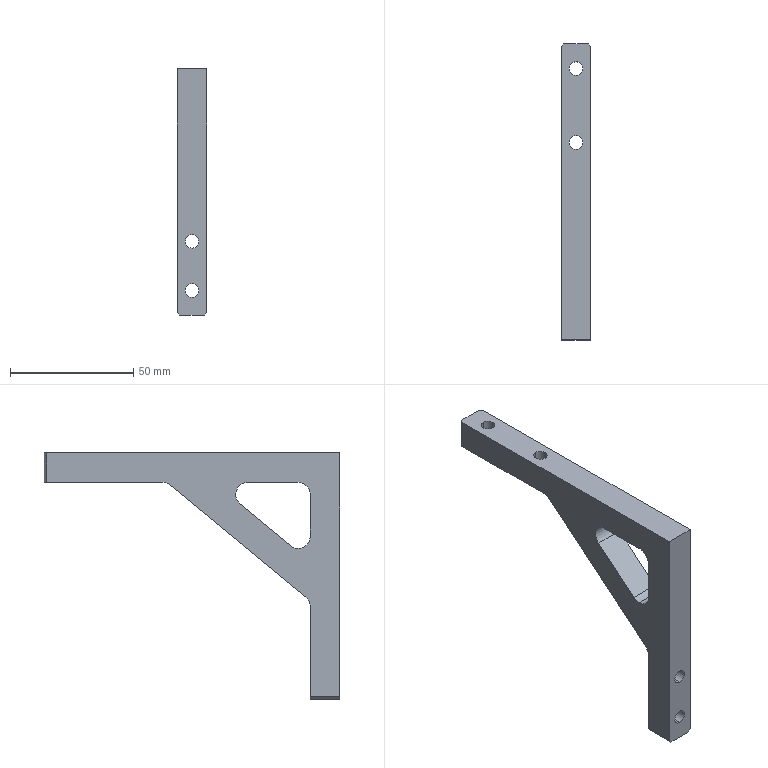Part | SolidWorks | features HoleWzd 2, Chamfer 1, Extrusion 1, Fillet 1, ICE 1 | 1 solid | 42 faces | box 12 x 120 x 100 mm | volume 37463 mm3 | cylinder 22 | plane 20 | commonest cylinder face diameters 10 x14 5.5 x8
STEP:
#1=CARTESIAN_POINT('',(6.,6.3,-95.));
#2=VERTEX_POINT('',#1);
#3=CARTESIAN_POINT('',(6.,6.3,-85.));
#4=VERTEX_POINT('',#3);
#5=CARTESIAN_POINT('',(6.,6.3,-90.));
#6=DIRECTION('',(0.,1.,0.));
#7=DIRECTION('',(0.,0.,1.));
#8=AXIS2_PLACEMENT_3D('',#5,#6,#7);
#9=CIRCLE('',#8,5.);
#10=EDGE_CURVE('',#2,#4,#9,.T.);
#11=ORIENTED_EDGE('',*,*,#10,.F.);
#12=CARTESIAN_POINT('',(6.,12.,-95.));
#13=VERTEX_POINT('',#12);
#14=CARTESIAN_POINT('',(6.,12.,-95.));
#15=DIRECTION('',(0.,1.,0.));
#16=VECTOR('',#15,1000.);
#17=LINE('',#14,#16);
#18=EDGE_CURVE('',#2,#13,#17,.T.);
#19=ORIENTED_EDGE('',*,*,#18,.T.);
#20=CARTESIAN_POINT('',(6.,12.,-85.));
#21=VERTEX_POINT('',#20);
#22=CARTESIAN_POINT('',(6.,12.,-90.));
#23=DIRECTION('',(0.,1.,0.));
#24=DIRECTION('',(0.,0.,1.));
#25=AXIS2_PLACEMENT_3D('',#22,#23,#24);
#26=CIRCLE('',#25,5.);
#27=EDGE_CURVE('',#13,#21,#26,.T.);
#28=ORIENTED_EDGE('',*,*,#27,.T.);
#29=CARTESIAN_POINT('',(6.,12.,-85.));
#30=DIRECTION('',(0.,1.,0.));
#31=VECTOR('',#30,1000.);
#32=LINE('',#29,#31);
#33=EDGE_CURVE('',#4,#21,#32,.T.);
#34=ORIENTED_EDGE('',*,*,#33,.F.);
#35=EDGE_LOOP('',(#11,#19,#28,#34));
#36=FACE_OUTER_BOUND('',#35,.T.);
#37=CARTESIAN_POINT('',(6.,12.,-90.));
#38=DIRECTION('',(0.,1.,0.));
#39=DIRECTION('',(0.,0.,1.));
#40=AXIS2_PLACEMENT_3D('',#37,#38,#39);
#41=CYLINDRICAL_SURFACE('',#40,5.);
#42=ADVANCED_FACE('',(#36),#41,.F.);
#43=CARTESIAN_POINT('',(6.,0.,-92.75));
#44=VERTEX_POINT('',#43);
#45=CARTESIAN_POINT('',(6.,0.,-87.25));
#46=VERTEX_POINT('',#45);
#47=CARTESIAN_POINT('',(6.,0.,-90.));
#48=DIRECTION('',(0.,1.,0.));
#49=DIRECTION('',(0.,0.,1.));
#50=AXIS2_PLACEMENT_3D('',#47,#48,#49);
#51=CIRCLE('',#50,2.75);
#52=EDGE_CURVE('',#44,#46,#51,.T.);
#53=ORIENTED_EDGE('',*,*,#52,.F.);
#54=CARTESIAN_POINT('',(6.,6.3,-92.75));
#55=VERTEX_POINT('',#54);
#56=CARTESIAN_POINT('',(6.,12.,-92.75));
#57=DIRECTION('',(0.,1.,0.));
#58=VECTOR('',#57,1000.);
#59=LINE('',#56,#58);
#60=EDGE_CURVE('',#44,#55,#59,.T.);
#61=ORIENTED_EDGE('',*,*,#60,.T.);
#62=CARTESIAN_POINT('',(6.,6.3,-87.25));
#63=VERTEX_POINT('',#62);
#64=CARTESIAN_POINT('',(6.,6.3,-90.));
#65=DIRECTION('',(0.,1.,0.));
#66=DIRECTION('',(0.,0.,1.));
#67=AXIS2_PLACEMENT_3D('',#64,#65,#66);
#68=CIRCLE('',#67,2.75);
#69=EDGE_CURVE('',#55,#63,#68,.T.);
#70=ORIENTED_EDGE('',*,*,#69,.T.);
#71=CARTESIAN_POINT('',(6.,12.,-87.25));
#72=DIRECTION('',(0.,1.,0.));
#73=VECTOR('',#72,1000.);
#74=LINE('',#71,#73);
#75=EDGE_CURVE('',#46,#63,#74,.T.);
#76=ORIENTED_EDGE('',*,*,#75,.F.);
#77=EDGE_LOOP('',(#53,#61,#70,#76));
#78=FACE_OUTER_BOUND('',#77,.T.);
#79=CARTESIAN_POINT('',(6.,12.,-90.));
#80=DIRECTION('',(0.,1.,0.));
#81=DIRECTION('',(0.,0.,1.));
#82=AXIS2_PLACEMENT_3D('',#79,#80,#81);
#83=CYLINDRICAL_SURFACE('',#82,2.75);
#84=ADVANCED_FACE('',(#78),#83,.F.);
#85=CARTESIAN_POINT('',(6.,6.3,-75.));
#86=VERTEX_POINT('',#85);
#87=CARTESIAN_POINT('',(6.,6.3,-65.));
#88=VERTEX_POINT('',#87);
#89=CARTESIAN_POINT('',(6.,6.3,-70.));
#90=DIRECTION('',(0.,1.,0.));
#91=DIRECTION('',(0.,0.,1.));
#92=AXIS2_PLACEMENT_3D('',#89,#90,#91);
#93=CIRCLE('',#92,5.);
#94=EDGE_CURVE('',#86,#88,#93,.T.);
#95=ORIENTED_EDGE('',*,*,#94,.F.);
#96=CARTESIAN_POINT('',(6.,12.,-75.));
#97=VERTEX_POINT('',#96);
#98=CARTESIAN_POINT('',(6.,12.,-75.));
#99=DIRECTION('',(0.,1.,0.));
#100=VECTOR('',#99,1000.);
#101=LINE('',#98,#100);
#102=EDGE_CURVE('',#86,#97,#101,.T.);
#103=ORIENTED_EDGE('',*,*,#102,.T.);
#104=CARTESIAN_POINT('',(6.,12.,-65.));
#105=VERTEX_POINT('',#104);
#106=CARTESIAN_POINT('',(6.,12.,-70.));
#107=DIRECTION('',(0.,1.,0.));
#108=DIRECTION('',(0.,0.,1.));
#109=AXIS2_PLACEMENT_3D('',#106,#107,#108);
#110=CIRCLE('',#109,5.);
#111=EDGE_CURVE('',#97,#105,#110,.T.);
#112=ORIENTED_EDGE('',*,*,#111,.T.);
#113=CARTESIAN_POINT('',(6.,12.,-65.));
#114=DIRECTION('',(0.,1.,0.));
#115=VECTOR('',#114,1000.);
#116=LINE('',#113,#115);
#117=EDGE_CURVE('',#88,#105,#116,.T.);
#118=ORIENTED_EDGE('',*,*,#117,.F.);
#119=EDGE_LOOP('',(#95,#103,#112,#118));
#120=FACE_OUTER_BOUND('',#119,.T.);
#121=CARTESIAN_POINT('',(6.,12.,-70.));
#122=DIRECTION('',(0.,1.,0.));
#123=DIRECTION('',(0.,0.,1.));
#124=AXIS2_PLACEMENT_3D('',#121,#122,#123);
#125=CYLINDRICAL_SURFACE('',#124,5.);
#126=ADVANCED_FACE('',(#120),#125,.F.);
#127=CARTESIAN_POINT('',(6.,0.,-72.75));
#128=VERTEX_POINT('',#127);
#129=CARTESIAN_POINT('',(6.,0.,-67.25));
#130=VERTEX_POINT('',#129);
#131=CARTESIAN_POINT('',(6.,0.,-70.));
#132=DIRECTION('',(0.,1.,0.));
#133=DIRECTION('',(0.,0.,1.));
#134=AXIS2_PLACEMENT_3D('',#131,#132,#133);
#135=CIRCLE('',#134,2.75);
#136=EDGE_CURVE('',#128,#130,#135,.T.);
#137=ORIENTED_EDGE('',*,*,#136,.F.);
#138=CARTESIAN_POINT('',(6.,6.3,-72.75));
#139=VERTEX_POINT('',#138);
#140=CARTESIAN_POINT('',(6.,12.,-72.75));
#141=DIRECTION('',(0.,1.,0.));
#142=VECTOR('',#141,1000.);
#143=LINE('',#140,#142);
#144=EDGE_CURVE('',#128,#139,#143,.T.);
#145=ORIENTED_EDGE('',*,*,#144,.T.);
#146=CARTESIAN_POINT('',(6.,6.3,-67.25));
#147=VERTEX_POINT('',#146);
#148=CARTESIAN_POINT('',(6.,6.3,-70.));
#149=DIRECTION('',(0.,1.,0.));
#150=DIRECTION('',(0.,0.,1.));
#151=AXIS2_PLACEMENT_3D('',#148,#149,#150);
#152=CIRCLE('',#151,2.75);
#153=EDGE_CURVE('',#139,#147,#152,.T.);
#154=ORIENTED_EDGE('',*,*,#153,.T.);
#155=CARTESIAN_POINT('',(6.,12.,-67.25));
#156=DIRECTION('',(0.,1.,0.));
#157=VECTOR('',#156,1000.);
#158=LINE('',#155,#157);
#159=EDGE_CURVE('',#130,#147,#158,.T.);
#160=ORIENTED_EDGE('',*,*,#159,.F.);
#161=EDGE_LOOP('',(#137,#145,#154,#160));
#162=FACE_OUTER_BOUND('',#161,.T.);
#163=CARTESIAN_POINT('',(6.,12.,-70.));
#164=DIRECTION('',(0.,1.,0.));
#165=DIRECTION('',(0.,0.,1.));
#166=AXIS2_PLACEMENT_3D('',#163,#164,#165);
#167=CYLINDRICAL_SURFACE('',#166,2.75);
#168=ADVANCED_FACE('',(#162),#167,.F.);
#169=CARTESIAN_POINT('',(6.,105.,-6.3));
#170=VERTEX_POINT('',#169);
#171=CARTESIAN_POINT('',(6.,115.,-6.3));
#172=VERTEX_POINT('',#171);
#173=CARTESIAN_POINT('',(6.,110.,-6.3));
#174=DIRECTION('',(0.,0.,-1.));
#175=DIRECTION('',(0.,1.,0.));
#176=AXIS2_PLACEMENT_3D('',#173,#174,#175);
#177=CIRCLE('',#176,5.);
#178=EDGE_CURVE('',#170,#172,#177,.T.);
#179=ORIENTED_EDGE('',*,*,#178,.F.);
#180=CARTESIAN_POINT('',(6.,105.,-12.));
#181=VERTEX_POINT('',#180);
#182=CARTESIAN_POINT('',(6.,105.,-12.));
#183=DIRECTION('',(0.,0.,-1.));
#184=VECTOR('',#183,1000.);
#185=LINE('',#182,#184);
#186=EDGE_CURVE('',#170,#181,#185,.T.);
#187=ORIENTED_EDGE('',*,*,#186,.T.);
#188=CARTESIAN_POINT('',(6.,115.,-12.));
#189=VERTEX_POINT('',#188);
#190=CARTESIAN_POINT('',(6.,110.,-12.));
#191=DIRECTION('',(0.,0.,-1.));
#192=DIRECTION('',(0.,1.,0.));
#193=AXIS2_PLACEMENT_3D('',#190,#191,#192);
#194=CIRCLE('',#193,5.);
#195=EDGE_CURVE('',#181,#189,#194,.T.);
#196=ORIENTED_EDGE('',*,*,#195,.T.);
#197=CARTESIAN_POINT('',(6.,115.,-12.));
#198=DIRECTION('',(0.,0.,-1.));
#199=VECTOR('',#198,1000.);
#200=LINE('',#197,#199);
#201=EDGE_CURVE('',#172,#189,#200,.T.);
#202=ORIENTED_EDGE('',*,*,#201,.F.);
#203=EDGE_LOOP('',(#179,#187,#196,#202));
#204=FACE_OUTER_BOUND('',#203,.T.);
#205=CARTESIAN_POINT('',(6.,110.,-12.));
#206=DIRECTION('',(0.,0.,-1.));
#207=DIRECTION('',(0.,1.,0.));
#208=AXIS2_PLACEMENT_3D('',#205,#206,#207);
#209=CYLINDRICAL_SURFACE('',#208,5.);
#210=ADVANCED_FACE('',(#204),#209,.F.);
#211=CARTESIAN_POINT('',(6.,107.25,0.));
#212=VERTEX_POINT('',#211);
#213=CARTESIAN_POINT('',(6.,112.75,0.));
#214=VERTEX_POINT('',#213);
#215=CARTESIAN_POINT('',(6.,110.,0.));
#216=DIRECTION('',(0.,0.,-1.));
#217=DIRECTION('',(0.,1.,0.));
#218=AXIS2_PLACEMENT_3D('',#215,#216,#217);
#219=CIRCLE('',#218,2.75);
#220=EDGE_CURVE('',#212,#214,#219,.T.);
#221=ORIENTED_EDGE('',*,*,#220,.F.);
#222=CARTESIAN_POINT('',(6.,107.25,-6.3));
#223=VERTEX_POINT('',#222);
#224=CARTESIAN_POINT('',(6.,107.25,-12.));
#225=DIRECTION('',(0.,0.,-1.));
#226=VECTOR('',#225,1000.);
#227=LINE('',#224,#226);
#228=EDGE_CURVE('',#212,#223,#227,.T.);
#229=ORIENTED_EDGE('',*,*,#228,.T.);
#230=CARTESIAN_POINT('',(6.,112.75,-6.3));
#231=VERTEX_POINT('',#230);
#232=CARTESIAN_POINT('',(6.,110.,-6.3));
#233=DIRECTION('',(0.,0.,-1.));
#234=DIRECTION('',(0.,1.,0.));
#235=AXIS2_PLACEMENT_3D('',#232,#233,#234);
#236=CIRCLE('',#235,2.75);
#237=EDGE_CURVE('',#223,#231,#236,.T.);
#238=ORIENTED_EDGE('',*,*,#237,.T.);
#239=CARTESIAN_POINT('',(6.,112.75,-12.));
#240=DIRECTION('',(0.,0.,-1.));
#241=VECTOR('',#240,1000.);
#242=LINE('',#239,#241);
#243=EDGE_CURVE('',#214,#231,#242,.T.);
#244=ORIENTED_EDGE('',*,*,#243,.F.);
#245=EDGE_LOOP('',(#221,#229,#238,#244));
#246=FACE_OUTER_BOUND('',#245,.T.);
#247=CARTESIAN_POINT('',(6.,110.,-12.));
#248=DIRECTION('',(0.,0.,-1.));
#249=DIRECTION('',(0.,1.,0.));
#250=AXIS2_PLACEMENT_3D('',#247,#248,#249);
#251=CYLINDRICAL_SURFACE('',#250,2.75);
#252=ADVANCED_FACE('',(#246),#251,.F.);
#253=CARTESIAN_POINT('',(6.,75.,-6.3));
#254=VERTEX_POINT('',#253);
#255=CARTESIAN_POINT('',(6.,85.,-6.3));
#256=VERTEX_POINT('',#255);
#257=CARTESIAN_POINT('',(6.,80.,-6.3));
#258=DIRECTION('',(0.,0.,-1.));
#259=DIRECTION('',(0.,1.,0.));
#260=AXIS2_PLACEMENT_3D('',#257,#258,#259);
#261=CIRCLE('',#260,5.);
#262=EDGE_CURVE('',#254,#256,#261,.T.);
#263=ORIENTED_EDGE('',*,*,#262,.F.);
#264=CARTESIAN_POINT('',(6.,75.,-12.));
#265=VERTEX_POINT('',#264);
#266=CARTESIAN_POINT('',(6.,75.,-12.));
#267=DIRECTION('',(0.,0.,-1.));
#268=VECTOR('',#267,1000.);
#269=LINE('',#266,#268);
#270=EDGE_CURVE('',#254,#265,#269,.T.);
#271=ORIENTED_EDGE('',*,*,#270,.T.);
#272=CARTESIAN_POINT('',(6.,85.,-12.));
#273=VERTEX_POINT('',#272);
#274=CARTESIAN_POINT('',(6.,80.,-12.));
#275=DIRECTION('',(0.,0.,-1.));
#276=DIRECTION('',(0.,1.,0.));
#277=AXIS2_PLACEMENT_3D('',#274,#275,#276);
#278=CIRCLE('',#277,5.);
#279=EDGE_CURVE('',#265,#273,#278,.T.);
#280=ORIENTED_EDGE('',*,*,#279,.T.);
#281=CARTESIAN_POINT('',(6.,85.,-12.));
#282=DIRECTION('',(0.,0.,-1.));
#283=VECTOR('',#282,1000.);
#284=LINE('',#281,#283);
#285=EDGE_CURVE('',#256,#273,#284,.T.);
#286=ORIENTED_EDGE('',*,*,#285,.F.);
#287=EDGE_LOOP('',(#263,#271,#280,#286));
#288=FACE_OUTER_BOUND('',#287,.T.);
#289=CARTESIAN_POINT('',(6.,80.,-12.));
#290=DIRECTION('',(0.,0.,-1.));
#291=DIRECTION('',(0.,1.,0.));
#292=AXIS2_PLACEMENT_3D('',#289,#290,#291);
#293=CYLINDRICAL_SURFACE('',#292,5.);
#294=ADVANCED_FACE('',(#288),#293,.F.);
#295=CARTESIAN_POINT('',(6.,77.25,0.));
#296=VERTEX_POINT('',#295);
#297=CARTESIAN_POINT('',(6.,82.75,0.));
#298=VERTEX_POINT('',#297);
#299=CARTESIAN_POINT('',(6.,80.,0.));
#300=DIRECTION('',(0.,0.,-1.));
#301=DIRECTION('',(0.,1.,0.));
#302=AXIS2_PLACEMENT_3D('',#299,#300,#301);
#303=CIRCLE('',#302,2.75);
#304=EDGE_CURVE('',#296,#298,#303,.T.);
#305=ORIENTED_EDGE('',*,*,#304,.F.);
#306=CARTESIAN_POINT('',(6.,77.25,-6.3));
#307=VERTEX_POINT('',#306);
#308=CARTESIAN_POINT('',(6.,77.25,-12.));
#309=DIRECTION('',(0.,0.,-1.));
#310=VECTOR('',#309,1000.);
#311=LINE('',#308,#310);
#312=EDGE_CURVE('',#296,#307,#311,.T.);
#313=ORIENTED_EDGE('',*,*,#312,.T.);
#314=CARTESIAN_POINT('',(6.,82.75,-6.3));
#315=VERTEX_POINT('',#314);
#316=CARTESIAN_POINT('',(6.,80.,-6.3));
#317=DIRECTION('',(0.,0.,-1.));
#318=DIRECTION('',(0.,1.,0.));
#319=AXIS2_PLACEMENT_3D('',#316,#317,#318);
#320=CIRCLE('',#319,2.75);
#321=EDGE_CURVE('',#307,#315,#320,.T.);
#322=ORIENTED_EDGE('',*,*,#321,.T.);
#323=CARTESIAN_POINT('',(6.,82.75,-12.));
#324=DIRECTION('',(0.,0.,-1.));
#325=VECTOR('',#324,1000.);
#326=LINE('',#323,#325);
#327=EDGE_CURVE('',#298,#315,#326,.T.);
#328=ORIENTED_EDGE('',*,*,#327,.F.);
#329=EDGE_LOOP('',(#305,#313,#322,#328));
#330=FACE_OUTER_BOUND('',#329,.T.);
#331=CARTESIAN_POINT('',(6.,80.,-12.));
#332=DIRECTION('',(0.,0.,-1.));
#333=DIRECTION('',(0.,1.,0.));
#334=AXIS2_PLACEMENT_3D('',#331,#332,#333);
#335=CYLINDRICAL_SURFACE('',#334,2.75);
#336=ADVANCED_FACE('',(#330),#335,.F.);
#337=CARTESIAN_POINT('',(0.,17.,-38.795));
#338=VERTEX_POINT('',#337);
#339=CARTESIAN_POINT('',(0.,20.188,-37.647));
#340=VERTEX_POINT('',#339);
#341=CARTESIAN_POINT('',(0.,17.,-33.795));
#342=DIRECTION('',(1.,0.,0.));
#343=DIRECTION('',(0.,0.,-1.));
#344=AXIS2_PLACEMENT_3D('',#341,#342,#343);
#345=CIRCLE('',#344,5.);
#346=EDGE_CURVE('',#338,#340,#345,.T.);
#347=ORIENTED_EDGE('',*,*,#346,.F.);
#348=CARTESIAN_POINT('',(12.,17.,-38.795));
#349=VERTEX_POINT('',#348);
#350=CARTESIAN_POINT('',(0.,17.,-38.795));
#351=DIRECTION('',(1.,0.,0.));
#352=VECTOR('',#351,1000.);
#353=LINE('',#350,#352);
#354=EDGE_CURVE('',#338,#349,#353,.T.);
#355=ORIENTED_EDGE('',*,*,#354,.T.);
#356=CARTESIAN_POINT('',(12.,20.188,-37.647));
#357=VERTEX_POINT('',#356);
#358=CARTESIAN_POINT('',(12.,17.,-33.795));
#359=DIRECTION('',(1.,0.,0.));
#360=DIRECTION('',(0.,0.,-1.));
#361=AXIS2_PLACEMENT_3D('',#358,#359,#360);
#362=CIRCLE('',#361,5.);
#363=EDGE_CURVE('',#349,#357,#362,.T.);
#364=ORIENTED_EDGE('',*,*,#363,.T.);
#365=CARTESIAN_POINT('',(0.,20.188,-37.647));
#366=DIRECTION('',(1.,0.,0.));
#367=VECTOR('',#366,1000.);
#368=LINE('',#365,#367);
#369=EDGE_CURVE('',#340,#357,#368,.T.);
#370=ORIENTED_EDGE('',*,*,#369,.F.);
#371=EDGE_LOOP('',(#347,#355,#364,#370));
#372=FACE_OUTER_BOUND('',#371,.T.);
#373=CARTESIAN_POINT('',(0.,17.,-33.795));
#374=DIRECTION('',(1.,0.,0.));
#375=DIRECTION('',(0.,0.,-1.));
#376=AXIS2_PLACEMENT_3D('',#373,#374,#375);
#377=CYLINDRICAL_SURFACE('',#376,5.);
#378=ADVANCED_FACE('',(#372),#377,.F.);
#379=CARTESIAN_POINT('',(6.,0.,-90.));
#380=DIRECTION('',(0.,1.,0.));
#381=DIRECTION('',(0.,0.,1.));
#382=AXIS2_PLACEMENT_3D('',#379,#380,#381);
#383=CIRCLE('',#382,2.75);
#384=EDGE_CURVE('',#46,#44,#383,.T.);
#385=ORIENTED_EDGE('',*,*,#384,.T.);
#386=ORIENTED_EDGE('',*,*,#52,.T.);
#387=EDGE_LOOP('',(#385,#386));
#388=FACE_BOUND('',#387,.T.);
#389=CARTESIAN_POINT('',(6.,0.,-70.));
#390=DIRECTION('',(0.,1.,0.));
#391=DIRECTION('',(0.,0.,1.));
#392=AXIS2_PLACEMENT_3D('',#389,#390,#391);
#393=CIRCLE('',#392,2.75);
#394=EDGE_CURVE('',#130,#128,#393,.T.);
#395=ORIENTED_EDGE('',*,*,#394,.T.);
#396=ORIENTED_EDGE('',*,*,#136,.T.);
#397=EDGE_LOOP('',(#395,#396));
#398=FACE_BOUND('',#397,.T.);
#399=CARTESIAN_POINT('',(11.,0.,-100.));
#400=VERTEX_POINT('',#399);
#401=CARTESIAN_POINT('',(1.,0.,-100.));
#402=VERTEX_POINT('',#401);
#403=CARTESIAN_POINT('',(12.,0.,-100.));
#404=DIRECTION('',(-1.,0.,0.));
#405=VECTOR('',#404,1000.);
#406=LINE('',#403,#405);
#407=EDGE_CURVE('',#400,#402,#406,.T.);
#408=ORIENTED_EDGE('',*,*,#407,.F.);
#409=CARTESIAN_POINT('',(12.,0.,-99.));
#410=VERTEX_POINT('',#409);
#411=CARTESIAN_POINT('',(12.,0.,-99.));
#412=DIRECTION('',(0.7071,0.,0.7071));
#413=VECTOR('',#412,1000.);
#414=LINE('',#411,#413);
#415=EDGE_CURVE('',#400,#410,#414,.T.);
#416=ORIENTED_EDGE('',*,*,#415,.T.);
#417=CARTESIAN_POINT('',(12.,0.,0.));
#418=VERTEX_POINT('',#417);
#419=CARTESIAN_POINT('',(12.,0.,-100.));
#420=DIRECTION('',(0.,0.,-1.));
#421=VECTOR('',#420,1000.);
#422=LINE('',#419,#421);
#423=EDGE_CURVE('',#418,#410,#422,.T.);
#424=ORIENTED_EDGE('',*,*,#423,.F.);
#425=CARTESIAN_POINT('',(0.,0.,0.));
#426=VERTEX_POINT('',#425);
#427=CARTESIAN_POINT('',(12.,0.,0.));
#428=DIRECTION('',(-1.,0.,0.));
#429=VECTOR('',#428,1000.);
#430=LINE('',#427,#429);
#431=EDGE_CURVE('',#418,#426,#430,.T.);
#432=ORIENTED_EDGE('',*,*,#431,.T.);
#433=CARTESIAN_POINT('',(0.,0.,-99.));
#434=VERTEX_POINT('',#433);
#435=CARTESIAN_POINT('',(0.,0.,-100.));
#436=DIRECTION('',(0.,0.,-1.));
#437=VECTOR('',#436,1000.);
#438=LINE('',#435,#437);
#439=EDGE_CURVE('',#426,#434,#438,.T.);
#440=ORIENTED_EDGE('',*,*,#439,.T.);
#441=CARTESIAN_POINT('',(1.,0.,-100.));
#442=DIRECTION('',(0.7071,0.,-0.7071));
#443=VECTOR('',#442,1000.);
#444=LINE('',#441,#443);
#445=EDGE_CURVE('',#434,#402,#444,.T.);
#446=ORIENTED_EDGE('',*,*,#445,.T.);
#447=EDGE_LOOP('',(#408,#416,#424,#432,#440,#446));
#448=FACE_OUTER_BOUND('',#447,.T.);
#449=CARTESIAN_POINT('',(12.,0.,-100.));
#450=DIRECTION('',(0.,1.,0.));
#451=DIRECTION('',(0.,0.,1.));
#452=AXIS2_PLACEMENT_3D('',#449,#450,#451);
#453=PLANE('',#452);
#454=ADVANCED_FACE('',(#388,#398,#448),#453,.F.);
#455=CARTESIAN_POINT('',(11.,12.,-100.));
#456=VERTEX_POINT('',#455);
#457=CARTESIAN_POINT('',(1.,12.,-100.));
#458=VERTEX_POINT('',#457);
#459=CARTESIAN_POINT('',(12.,12.,-100.));
#460=DIRECTION('',(-1.,0.,0.));
#461=VECTOR('',#460,1000.);
#462=LINE('',#459,#461);
#463=EDGE_CURVE('',#456,#458,#462,.T.);
#464=ORIENTED_EDGE('',*,*,#463,.F.);
#465=CARTESIAN_POINT('',(11.,12.,-100.));
#466=DIRECTION('',(0.,-1.,0.));
#467=VECTOR('',#466,1000.);
#468=LINE('',#465,#467);
#469=EDGE_CURVE('',#456,#400,#468,.T.);
#470=ORIENTED_EDGE('',*,*,#469,.T.);
#471=ORIENTED_EDGE('',*,*,#407,.T.);
#472=CARTESIAN_POINT('',(1.,12.,-100.));
#473=DIRECTION('',(0.,1.,0.));
#474=VECTOR('',#473,1000.);
#475=LINE('',#472,#474);
#476=EDGE_CURVE('',#402,#458,#475,.T.);
#477=ORIENTED_EDGE('',*,*,#476,.T.);
#478=EDGE_LOOP('',(#464,#470,#471,#477));
#479=FACE_OUTER_BOUND('',#478,.T.);
#480=CARTESIAN_POINT('',(12.,12.,-100.));
#481=DIRECTION('',(0.,0.,1.));
#482=DIRECTION('',(1.,0.,0.));
#483=AXIS2_PLACEMENT_3D('',#480,#481,#482);
#484=PLANE('',#483);
#485=ADVANCED_FACE('',(#479),#484,.F.);
#486=CARTESIAN_POINT('',(6.,12.,-90.));
#487=DIRECTION('',(0.,1.,0.));
#488=DIRECTION('',(0.,0.,1.));
#489=AXIS2_PLACEMENT_3D('',#486,#487,#488);
#490=CIRCLE('',#489,5.);
#491=EDGE_CURVE('',#21,#13,#490,.T.);
#492=ORIENTED_EDGE('',*,*,#491,.F.);
#493=ORIENTED_EDGE('',*,*,#27,.F.);
#494=EDGE_LOOP('',(#492,#493));
#495=FACE_BOUND('',#494,.T.);
#496=CARTESIAN_POINT('',(6.,12.,-70.));
#497=DIRECTION('',(0.,1.,0.));
#498=DIRECTION('',(0.,0.,1.));
#499=AXIS2_PLACEMENT_3D('',#496,#497,#498);
#500=CIRCLE('',#499,5.);
#501=EDGE_CURVE('',#105,#97,#500,.T.);
#502=ORIENTED_EDGE('',*,*,#501,.F.);
#503=ORIENTED_EDGE('',*,*,#111,.F.);
#504=EDGE_LOOP('',(#502,#503));
#505=FACE_BOUND('',#504,.T.);
#506=CARTESIAN_POINT('',(0.,12.,-99.));
#507=VERTEX_POINT('',#506);
#508=CARTESIAN_POINT('',(0.,12.,-62.352));
#509=VERTEX_POINT('',#508);
#510=CARTESIAN_POINT('',(0.,12.,-60.));
#511=DIRECTION('',(0.,0.,1.));
#512=VECTOR('',#511,1000.);
#513=LINE('',#510,#512);
#514=EDGE_CURVE('',#507,#509,#513,.T.);
#515=ORIENTED_EDGE('',*,*,#514,.T.);
#516=CARTESIAN_POINT('',(12.,12.,-62.352));
#517=VERTEX_POINT('',#516);
#518=CARTESIAN_POINT('',(12.,12.,-62.352));
#519=DIRECTION('',(1.,0.,0.));
#520=VECTOR('',#519,1000.);
#521=LINE('',#518,#520);
#522=EDGE_CURVE('',#509,#517,#521,.T.);
#523=ORIENTED_EDGE('',*,*,#522,.T.);
#524=CARTESIAN_POINT('',(12.,12.,-99.));
#525=VERTEX_POINT('',#524);
#526=CARTESIAN_POINT('',(12.,12.,-60.));
#527=DIRECTION('',(0.,0.,1.));
#528=VECTOR('',#527,1000.);
#529=LINE('',#526,#528);
#530=EDGE_CURVE('',#525,#517,#529,.T.);
#531=ORIENTED_EDGE('',*,*,#530,.F.);
#532=CARTESIAN_POINT('',(12.,12.,-99.));
#533=DIRECTION('',(-0.7071,0.,-0.7071));
#534=VECTOR('',#533,1000.);
#535=LINE('',#532,#534);
#536=EDGE_CURVE('',#525,#456,#535,.T.);
#537=ORIENTED_EDGE('',*,*,#536,.T.);
#538=ORIENTED_EDGE('',*,*,#463,.T.);
#539=CARTESIAN_POINT('',(1.,12.,-100.));
#540=DIRECTION('',(-0.7071,0.,0.7071));
#541=VECTOR('',#540,1000.);
#542=LINE('',#539,#541);
#543=EDGE_CURVE('',#458,#507,#542,.T.);
#544=ORIENTED_EDGE('',*,*,#543,.T.);
#545=EDGE_LOOP('',(#515,#523,#531,#537,#538,#544));
#546=FACE_OUTER_BOUND('',#545,.T.);
#547=CARTESIAN_POINT('',(12.,12.,-60.));
#548=DIRECTION('',(0.,-1.,0.));
#549=DIRECTION('',(0.,0.,-1.));
#550=AXIS2_PLACEMENT_3D('',#547,#548,#549);
#551=PLANE('',#550);
#552=ADVANCED_FACE('',(#495,#505,#546),#551,.F.);
#553=CARTESIAN_POINT('',(12.,13.812,-58.5));
#554=VERTEX_POINT('',#553);
#555=CARTESIAN_POINT('',(12.,68.613,-13.148));
#556=VERTEX_POINT('',#555);
#557=CARTESIAN_POINT('',(12.,70.,-12.));
#558=DIRECTION('',(0.,0.7704,0.6376));
#559=VECTOR('',#558,1000.);
#560=LINE('',#557,#559);
#561=EDGE_CURVE('',#554,#556,#560,.T.);
#562=ORIENTED_EDGE('',*,*,#561,.F.);
#563=CARTESIAN_POINT('',(0.,13.812,-58.5));
#564=VERTEX_POINT('',#563);
#565=CARTESIAN_POINT('',(0.,13.812,-58.5));
#566=DIRECTION('',(-1.,0.,0.));
#567=VECTOR('',#566,1000.);
#568=LINE('',#565,#567);
#569=EDGE_CURVE('',#554,#564,#568,.T.);
#570=ORIENTED_EDGE('',*,*,#569,.T.);
#571=CARTESIAN_POINT('',(0.,68.613,-13.148));
#572=VERTEX_POINT('',#571);
#573=CARTESIAN_POINT('',(0.,70.,-12.));
#574=DIRECTION('',(0.,0.7704,0.6376));
#575=VECTOR('',#574,1000.);
#576=LINE('',#573,#575);
#577=EDGE_CURVE('',#564,#572,#576,.T.);
#578=ORIENTED_EDGE('',*,*,#577,.T.);
#579=CARTESIAN_POINT('',(12.,68.613,-13.148));
#580=DIRECTION('',(1.,0.,0.));
#581=VECTOR('',#580,1000.);
#582=LINE('',#579,#581);
#583=EDGE_CURVE('',#572,#556,#582,.T.);
#584=ORIENTED_EDGE('',*,*,#583,.T.);
#585=EDGE_LOOP('',(#562,#570,#578,#584));
#586=FACE_OUTER_BOUND('',#585,.T.);
#587=CARTESIAN_POINT('',(12.,70.,-12.));
#588=DIRECTION('',(0.,-0.6376,0.7704));
#589=DIRECTION('',(0.,-0.7704,-0.6376));
#590=AXIS2_PLACEMENT_3D('',#587,#588,#589);
#591=PLANE('',#590);
#592=ADVANCED_FACE('',(#586),#591,.F.);
#593=CARTESIAN_POINT('',(6.,110.,-12.));
#594=DIRECTION('',(0.,0.,-1.));
#595=DIRECTION('',(0.,1.,0.));
#596=AXIS2_PLACEMENT_3D('',#593,#594,#595);
#597=CIRCLE('',#596,5.);
#598=EDGE_CURVE('',#189,#181,#597,.T.);
#599=ORIENTED_EDGE('',*,*,#598,.F.);
#600=ORIENTED_EDGE('',*,*,#195,.F.);
#601=EDGE_LOOP('',(#599,#600));
#602=FACE_BOUND('',#601,.T.);
#603=CARTESIAN_POINT('',(6.,80.,-12.));
#604=DIRECTION('',(0.,0.,-1.));
#605=DIRECTION('',(0.,1.,0.));
#606=AXIS2_PLACEMENT_3D('',#603,#604,#605);
#607=CIRCLE('',#606,5.);
#608=EDGE_CURVE('',#273,#265,#607,.T.);
#609=ORIENTED_EDGE('',*,*,#608,.F.);
#610=ORIENTED_EDGE('',*,*,#279,.F.);
#611=EDGE_LOOP('',(#609,#610));
#612=FACE_BOUND('',#611,.T.);
#613=CARTESIAN_POINT('',(12.,71.801,-12.));
#614=VERTEX_POINT('',#613);
#615=CARTESIAN_POINT('',(12.,119.,-12.));
#616=VERTEX_POINT('',#615);
#617=CARTESIAN_POINT('',(12.,120.,-12.));
#618=DIRECTION('',(0.,1.,0.));
#619=VECTOR('',#618,1000.);
#620=LINE('',#617,#619);
#621=EDGE_CURVE('',#614,#616,#620,.T.);
#622=ORIENTED_EDGE('',*,*,#621,.F.);
#623=CARTESIAN_POINT('',(0.,71.801,-12.));
#624=VERTEX_POINT('',#623);
#625=CARTESIAN_POINT('',(0.,71.801,-12.));
#626=DIRECTION('',(-1.,0.,0.));
#627=VECTOR('',#626,1000.);
#628=LINE('',#625,#627);
#629=EDGE_CURVE('',#614,#624,#628,.T.);
#630=ORIENTED_EDGE('',*,*,#629,.T.);
#631=CARTESIAN_POINT('',(0.,119.,-12.));
#632=VERTEX_POINT('',#631);
#633=CARTESIAN_POINT('',(0.,120.,-12.));
#634=DIRECTION('',(0.,1.,0.));
#635=VECTOR('',#634,1000.);
#636=LINE('',#633,#635);
#637=EDGE_CURVE('',#624,#632,#636,.T.);
#638=ORIENTED_EDGE('',*,*,#637,.T.);
#639=CARTESIAN_POINT('',(1.,120.,-12.));
#640=VERTEX_POINT('',#639);
#641=CARTESIAN_POINT('',(1.,120.,-12.));
#642=DIRECTION('',(0.7071,0.7071,0.));
#643=VECTOR('',#642,1000.);
#644=LINE('',#641,#643);
#645=EDGE_CURVE('',#632,#640,#644,.T.);
#646=ORIENTED_EDGE('',*,*,#645,.T.);
#647=CARTESIAN_POINT('',(11.,120.,-12.));
#648=VERTEX_POINT('',#647);
#649=CARTESIAN_POINT('',(12.,120.,-12.));
#650=DIRECTION('',(-1.,0.,0.));
#651=VECTOR('',#650,1000.);
#652=LINE('',#649,#651);
#653=EDGE_CURVE('',#648,#640,#652,.T.);
#654=ORIENTED_EDGE('',*,*,#653,.F.);
#655=CARTESIAN_POINT('',(12.,119.,-12.));
#656=DIRECTION('',(0.7071,-0.7071,0.));
#657=VECTOR('',#656,1000.);
#658=LINE('',#655,#657);
#659=EDGE_CURVE('',#648,#616,#658,.T.);
#660=ORIENTED_EDGE('',*,*,#659,.T.);
#661=EDGE_LOOP('',(#622,#630,#638,#646,#654,#660));
#662=FACE_OUTER_BOUND('',#661,.T.);
#663=CARTESIAN_POINT('',(12.,120.,-12.));
#664=DIRECTION('',(0.,0.,1.));
#665=DIRECTION('',(0.,-1.,0.));
#666=AXIS2_PLACEMENT_3D('',#663,#664,#665);
#667=PLANE('',#666);
#668=ADVANCED_FACE('',(#602,#612,#662),#667,.F.);
#669=CARTESIAN_POINT('',(11.,120.,0.));
#670=VERTEX_POINT('',#669);
#671=CARTESIAN_POINT('',(1.,120.,0.));
#672=VERTEX_POINT('',#671);
#673=CARTESIAN_POINT('',(12.,120.,0.));
#674=DIRECTION('',(-1.,0.,0.));
#675=VECTOR('',#674,1000.);
#676=LINE('',#673,#675);
#677=EDGE_CURVE('',#670,#672,#676,.T.);
#678=ORIENTED_EDGE('',*,*,#677,.F.);
#679=CARTESIAN_POINT('',(11.,120.,0.));
#680=DIRECTION('',(0.,0.,-1.));
#681=VECTOR('',#680,1000.);
#682=LINE('',#679,#681);
#683=EDGE_CURVE('',#670,#648,#682,.T.);
#684=ORIENTED_EDGE('',*,*,#683,.T.);
#685=ORIENTED_EDGE('',*,*,#653,.T.);
#686=CARTESIAN_POINT('',(1.,120.,0.));
#687=DIRECTION('',(0.,0.,1.));
#688=VECTOR('',#687,1000.);
#689=LINE('',#686,#688);
#690=EDGE_CURVE('',#640,#672,#689,.T.);
#691=ORIENTED_EDGE('',*,*,#690,.T.);
#692=EDGE_LOOP('',(#678,#684,#685,#691));
#693=FACE_OUTER_BOUND('',#692,.T.);
#694=CARTESIAN_POINT('',(12.,120.,0.));
#695=DIRECTION('',(0.,-1.,0.));
#696=DIRECTION('',(0.,0.,-1.));
#697=AXIS2_PLACEMENT_3D('',#694,#695,#696);
#698=PLANE('',#697);
#699=ADVANCED_FACE('',(#693),#698,.F.);
#700=CARTESIAN_POINT('',(6.,110.,0.));
#701=DIRECTION('',(0.,0.,-1.));
#702=DIRECTION('',(0.,1.,0.));
#703=AXIS2_PLACEMENT_3D('',#700,#701,#702);
#704=CIRCLE('',#703,2.75);
#705=EDGE_CURVE('',#214,#212,#704,.T.);
#706=ORIENTED_EDGE('',*,*,#705,.T.);
#707=ORIENTED_EDGE('',*,*,#220,.T.);
#708=EDGE_LOOP('',(#706,#707));
#709=FACE_BOUND('',#708,.T.);
#710=CARTESIAN_POINT('',(6.,80.,0.));
#711=DIRECTION('',(0.,0.,-1.));
#712=DIRECTION('',(0.,1.,0.));
#713=AXIS2_PLACEMENT_3D('',#710,#711,#712);
#714=CIRCLE('',#713,2.75);
#715=EDGE_CURVE('',#298,#296,#714,.T.);
#716=ORIENTED_EDGE('',*,*,#715,.T.);
#717=ORIENTED_EDGE('',*,*,#304,.T.);
#718=EDGE_LOOP('',(#716,#717));
#719=FACE_BOUND('',#718,.T.);
#720=CARTESIAN_POINT('',(12.,119.,0.));
#721=VERTEX_POINT('',#720);
#722=CARTESIAN_POINT('',(12.,0.,0.));
#723=DIRECTION('',(0.,-1.,0.));
#724=VECTOR('',#723,1000.);
#725=LINE('',#722,#724);
#726=EDGE_CURVE('',#721,#418,#725,.T.);
#727=ORIENTED_EDGE('',*,*,#726,.F.);
#728=CARTESIAN_POINT('',(12.,119.,0.));
#729=DIRECTION('',(-0.7071,0.7071,0.));
#730=VECTOR('',#729,1000.);
#731=LINE('',#728,#730);
#732=EDGE_CURVE('',#721,#670,#731,.T.);
#733=ORIENTED_EDGE('',*,*,#732,.T.);
#734=ORIENTED_EDGE('',*,*,#677,.T.);
#735=CARTESIAN_POINT('',(0.,119.,0.));
#736=VERTEX_POINT('',#735);
#737=CARTESIAN_POINT('',(1.,120.,0.));
#738=DIRECTION('',(-0.7071,-0.7071,0.));
#739=VECTOR('',#738,1000.);
#740=LINE('',#737,#739);
#741=EDGE_CURVE('',#672,#736,#740,.T.);
#742=ORIENTED_EDGE('',*,*,#741,.T.);
#743=CARTESIAN_POINT('',(0.,0.,0.));
#744=DIRECTION('',(0.,-1.,0.));
#745=VECTOR('',#744,1000.);
#746=LINE('',#743,#745);
#747=EDGE_CURVE('',#736,#426,#746,.T.);
#748=ORIENTED_EDGE('',*,*,#747,.T.);
#749=ORIENTED_EDGE('',*,*,#431,.F.);
#750=EDGE_LOOP('',(#727,#733,#734,#742,#748,#749));
#751=FACE_OUTER_BOUND('',#750,.T.);
#752=CARTESIAN_POINT('',(12.,0.,0.));
#753=DIRECTION('',(0.,0.,-1.));
#754=DIRECTION('',(-1.,0.,0.));
#755=AXIS2_PLACEMENT_3D('',#752,#753,#754);
#756=PLANE('',#755);
#757=ADVANCED_FACE('',(#709,#719,#751),#756,.F.);
#758=CARTESIAN_POINT('',(12.,40.482,-20.852));
#759=VERTEX_POINT('',#758);
#760=CARTESIAN_POINT('',(12.,20.188,-37.647));
#761=DIRECTION('',(0.,0.7704,0.6376));
#762=VECTOR('',#761,1000.);
#763=LINE('',#760,#762);
#764=EDGE_CURVE('',#357,#759,#763,.T.);
#765=ORIENTED_EDGE('',*,*,#764,.F.);
#766=ORIENTED_EDGE('',*,*,#363,.F.);
#767=CARTESIAN_POINT('',(12.,12.,-33.795));
#768=VERTEX_POINT('',#767);
#769=CARTESIAN_POINT('',(12.,17.,-33.795));
#770=DIRECTION('',(1.,0.,0.));
#771=DIRECTION('',(0.,0.,-1.));
#772=AXIS2_PLACEMENT_3D('',#769,#770,#771);
#773=CIRCLE('',#772,5.);
#774=EDGE_CURVE('',#768,#349,#773,.T.);
#775=ORIENTED_EDGE('',*,*,#774,.F.);
#776=CARTESIAN_POINT('',(12.,12.,-17.));
#777=VERTEX_POINT('',#776);
#778=CARTESIAN_POINT('',(12.,12.,-17.));
#779=DIRECTION('',(0.,0.,-1.));
#780=VECTOR('',#779,1000.);
#781=LINE('',#778,#780);
#782=EDGE_CURVE('',#777,#768,#781,.T.);
#783=ORIENTED_EDGE('',*,*,#782,.F.);
#784=CARTESIAN_POINT('',(12.,17.,-12.));
#785=VERTEX_POINT('',#784);
#786=CARTESIAN_POINT('',(12.,17.,-17.));
#787=DIRECTION('',(1.,0.,0.));
#788=DIRECTION('',(0.,0.,-1.));
#789=AXIS2_PLACEMENT_3D('',#786,#787,#788);
#790=CIRCLE('',#789,5.);
#791=EDGE_CURVE('',#785,#777,#790,.T.);
#792=ORIENTED_EDGE('',*,*,#791,.F.);
#793=CARTESIAN_POINT('',(12.,37.294,-12.));
#794=VERTEX_POINT('',#793);
#795=CARTESIAN_POINT('',(12.,37.294,-12.));
#796=DIRECTION('',(0.,-1.,0.));
#797=VECTOR('',#796,1000.);
#798=LINE('',#795,#797);
#799=EDGE_CURVE('',#794,#785,#798,.T.);
#800=ORIENTED_EDGE('',*,*,#799,.F.);
#801=CARTESIAN_POINT('',(12.,37.294,-17.));
#802=DIRECTION('',(1.,0.,0.));
#803=DIRECTION('',(0.,0.,1.));
#804=AXIS2_PLACEMENT_3D('',#801,#802,#803);
#805=CIRCLE('',#804,5.);
#806=EDGE_CURVE('',#759,#794,#805,.T.);
#807=ORIENTED_EDGE('',*,*,#806,.F.);
#808=EDGE_LOOP('',(#765,#766,#775,#783,#792,#800,#807));
#809=FACE_BOUND('',#808,.T.);
#810=ORIENTED_EDGE('',*,*,#561,.T.);
#811=CARTESIAN_POINT('',(12.,71.801,-17.));
#812=DIRECTION('',(-1.,0.,0.));
#813=DIRECTION('',(0.,0.,1.));
#814=AXIS2_PLACEMENT_3D('',#811,#812,#813);
#815=CIRCLE('',#814,5.);
#816=EDGE_CURVE('',#556,#614,#815,.T.);
#817=ORIENTED_EDGE('',*,*,#816,.T.);
#818=ORIENTED_EDGE('',*,*,#621,.T.);
#819=CARTESIAN_POINT('',(12.,119.,0.));
#820=DIRECTION('',(0.,0.,1.));
#821=VECTOR('',#820,1000.);
#822=LINE('',#819,#821);
#823=EDGE_CURVE('',#616,#721,#822,.T.);
#824=ORIENTED_EDGE('',*,*,#823,.T.);
#825=ORIENTED_EDGE('',*,*,#726,.T.);
#826=ORIENTED_EDGE('',*,*,#423,.T.);
#827=CARTESIAN_POINT('',(12.,0.,-99.));
#828=DIRECTION('',(0.,1.,0.));
#829=VECTOR('',#828,1000.);
#830=LINE('',#827,#829);
#831=EDGE_CURVE('',#410,#525,#830,.T.);
#832=ORIENTED_EDGE('',*,*,#831,.T.);
#833=ORIENTED_EDGE('',*,*,#530,.T.);
#834=CARTESIAN_POINT('',(12.,17.,-62.352));
#835=DIRECTION('',(-1.,0.,0.));
#836=DIRECTION('',(0.,0.,1.));
#837=AXIS2_PLACEMENT_3D('',#834,#835,#836);
#838=CIRCLE('',#837,5.);
#839=EDGE_CURVE('',#517,#554,#838,.T.);
#840=ORIENTED_EDGE('',*,*,#839,.T.);
#841=EDGE_LOOP('',(#810,#817,#818,#824,#825,#826,#832,#833,#840));
#842=FACE_OUTER_BOUND('',#841,.T.);
#843=CARTESIAN_POINT('',(12.,0.,0.));
#844=DIRECTION('',(-1.,0.,0.));
#845=DIRECTION('',(0.,0.,1.));
#846=AXIS2_PLACEMENT_3D('',#843,#844,#845);
#847=PLANE('',#846);
#848=ADVANCED_FACE('',(#809,#842),#847,.F.);
#849=CARTESIAN_POINT('',(0.,12.,-33.795));
#850=VERTEX_POINT('',#849);
#851=CARTESIAN_POINT('',(0.,17.,-33.795));
#852=DIRECTION('',(1.,0.,0.));
#853=DIRECTION('',(0.,0.,-1.));
#854=AXIS2_PLACEMENT_3D('',#851,#852,#853);
#855=CIRCLE('',#854,5.);
#856=EDGE_CURVE('',#850,#338,#855,.T.);
#857=ORIENTED_EDGE('',*,*,#856,.T.);
#858=ORIENTED_EDGE('',*,*,#346,.T.);
#859=CARTESIAN_POINT('',(0.,40.482,-20.852));
#860=VERTEX_POINT('',#859);
#861=CARTESIAN_POINT('',(0.,20.188,-37.647));
#862=DIRECTION('',(0.,0.7704,0.6376));
#863=VECTOR('',#862,1000.);
#864=LINE('',#861,#863);
#865=EDGE_CURVE('',#340,#860,#864,.T.);
#866=ORIENTED_EDGE('',*,*,#865,.T.);
#867=CARTESIAN_POINT('',(0.,37.294,-12.));
#868=VERTEX_POINT('',#867);
#869=CARTESIAN_POINT('',(0.,37.294,-17.));
#870=DIRECTION('',(1.,0.,0.));
#871=DIRECTION('',(0.,0.,1.));
#872=AXIS2_PLACEMENT_3D('',#869,#870,#871);
#873=CIRCLE('',#872,5.);
#874=EDGE_CURVE('',#860,#868,#873,.T.);
#875=ORIENTED_EDGE('',*,*,#874,.T.);
#876=CARTESIAN_POINT('',(0.,17.,-12.));
#877=VERTEX_POINT('',#876);
#878=CARTESIAN_POINT('',(0.,37.294,-12.));
#879=DIRECTION('',(0.,-1.,0.));
#880=VECTOR('',#879,1000.);
#881=LINE('',#878,#880);
#882=EDGE_CURVE('',#868,#877,#881,.T.);
#883=ORIENTED_EDGE('',*,*,#882,.T.);
#884=CARTESIAN_POINT('',(0.,12.,-17.));
#885=VERTEX_POINT('',#884);
#886=CARTESIAN_POINT('',(0.,17.,-17.));
#887=DIRECTION('',(1.,0.,0.));
#888=DIRECTION('',(0.,0.,-1.));
#889=AXIS2_PLACEMENT_3D('',#886,#887,#888);
#890=CIRCLE('',#889,5.);
#891=EDGE_CURVE('',#877,#885,#890,.T.);
#892=ORIENTED_EDGE('',*,*,#891,.T.);
#893=CARTESIAN_POINT('',(0.,12.,-17.));
#894=DIRECTION('',(0.,0.,-1.));
#895=VECTOR('',#894,1000.);
#896=LINE('',#893,#895);
#897=EDGE_CURVE('',#885,#850,#896,.T.);
#898=ORIENTED_EDGE('',*,*,#897,.T.);
#899=EDGE_LOOP('',(#857,#858,#866,#875,#883,#892,#898));
#900=FACE_BOUND('',#899,.T.);
#901=ORIENTED_EDGE('',*,*,#747,.F.);
#902=CARTESIAN_POINT('',(0.,119.,-12.));
#903=DIRECTION('',(0.,0.,-1.));
#904=VECTOR('',#903,1000.);
#905=LINE('',#902,#904);
#906=EDGE_CURVE('',#736,#632,#905,.T.);
#907=ORIENTED_EDGE('',*,*,#906,.T.);
#908=ORIENTED_EDGE('',*,*,#637,.F.);
#909=CARTESIAN_POINT('',(0.,71.801,-17.));
#910=DIRECTION('',(1.,0.,0.));
#911=DIRECTION('',(0.,0.,1.));
#912=AXIS2_PLACEMENT_3D('',#909,#910,#911);
#913=CIRCLE('',#912,5.);
#914=EDGE_CURVE('',#624,#572,#913,.T.);
#915=ORIENTED_EDGE('',*,*,#914,.T.);
#916=ORIENTED_EDGE('',*,*,#577,.F.);
#917=CARTESIAN_POINT('',(0.,17.,-62.352));
#918=DIRECTION('',(1.,0.,0.));
#919=DIRECTION('',(0.,0.,1.));
#920=AXIS2_PLACEMENT_3D('',#917,#918,#919);
#921=CIRCLE('',#920,5.);
#922=EDGE_CURVE('',#564,#509,#921,.T.);
#923=ORIENTED_EDGE('',*,*,#922,.T.);
#924=ORIENTED_EDGE('',*,*,#514,.F.);
#925=CARTESIAN_POINT('',(0.,0.,-99.));
#926=DIRECTION('',(0.,-1.,0.));
#927=VECTOR('',#926,1000.);
#928=LINE('',#925,#927);
#929=EDGE_CURVE('',#507,#434,#928,.T.);
#930=ORIENTED_EDGE('',*,*,#929,.T.);
#931=ORIENTED_EDGE('',*,*,#439,.F.);
#932=EDGE_LOOP('',(#901,#907,#908,#915,#916,#923,#924,#930,#931));
#933=FACE_OUTER_BOUND('',#932,.T.);
#934=CARTESIAN_POINT('',(0.,0.,0.));
#935=DIRECTION('',(-1.,0.,0.));
#936=DIRECTION('',(0.,0.,1.));
#937=AXIS2_PLACEMENT_3D('',#934,#935,#936);
#938=PLANE('',#937);
#939=ADVANCED_FACE('',(#900,#933),#938,.T.);
#940=ORIENTED_EDGE('',*,*,#354,.F.);
#941=ORIENTED_EDGE('',*,*,#856,.F.);
#942=CARTESIAN_POINT('',(0.,12.,-33.795));
#943=DIRECTION('',(1.,0.,0.));
#944=VECTOR('',#943,1000.);
#945=LINE('',#942,#944);
#946=EDGE_CURVE('',#850,#768,#945,.T.);
#947=ORIENTED_EDGE('',*,*,#946,.T.);
#948=ORIENTED_EDGE('',*,*,#774,.T.);
#949=EDGE_LOOP('',(#940,#941,#947,#948));
#950=FACE_OUTER_BOUND('',#949,.T.);
#951=CARTESIAN_POINT('',(0.,17.,-33.795));
#952=DIRECTION('',(1.,0.,0.));
#953=DIRECTION('',(0.,0.,-1.));
#954=AXIS2_PLACEMENT_3D('',#951,#952,#953);
#955=CYLINDRICAL_SURFACE('',#954,5.);
#956=ADVANCED_FACE('',(#950),#955,.F.);
#957=ORIENTED_EDGE('',*,*,#782,.T.);
#958=ORIENTED_EDGE('',*,*,#946,.F.);
#959=ORIENTED_EDGE('',*,*,#897,.F.);
#960=CARTESIAN_POINT('',(0.,12.,-17.));
#961=DIRECTION('',(1.,0.,0.));
#962=VECTOR('',#961,1000.);
#963=LINE('',#960,#962);
#964=EDGE_CURVE('',#885,#777,#963,.T.);
#965=ORIENTED_EDGE('',*,*,#964,.T.);
#966=EDGE_LOOP('',(#957,#958,#959,#965));
#967=FACE_OUTER_BOUND('',#966,.T.);
#968=CARTESIAN_POINT('',(0.,12.,-17.));
#969=DIRECTION('',(0.,-1.,0.));
#970=DIRECTION('',(0.,0.,-1.));
#971=AXIS2_PLACEMENT_3D('',#968,#969,#970);
#972=PLANE('',#971);
#973=ADVANCED_FACE('',(#967),#972,.F.);
#974=ORIENTED_EDGE('',*,*,#791,.T.);
#975=ORIENTED_EDGE('',*,*,#964,.F.);
#976=ORIENTED_EDGE('',*,*,#891,.F.);
#977=CARTESIAN_POINT('',(0.,17.,-12.));
#978=DIRECTION('',(1.,0.,0.));
#979=VECTOR('',#978,1000.);
#980=LINE('',#977,#979);
#981=EDGE_CURVE('',#877,#785,#980,.T.);
#982=ORIENTED_EDGE('',*,*,#981,.T.);
#983=EDGE_LOOP('',(#974,#975,#976,#982));
#984=FACE_OUTER_BOUND('',#983,.T.);
#985=CARTESIAN_POINT('',(0.,17.,-17.));
#986=DIRECTION('',(1.,0.,0.));
#987=DIRECTION('',(0.,0.,-1.));
#988=AXIS2_PLACEMENT_3D('',#985,#986,#987);
#989=CYLINDRICAL_SURFACE('',#988,5.);
#990=ADVANCED_FACE('',(#984),#989,.F.);
#991=ORIENTED_EDGE('',*,*,#799,.T.);
#992=ORIENTED_EDGE('',*,*,#981,.F.);
#993=ORIENTED_EDGE('',*,*,#882,.F.);
#994=CARTESIAN_POINT('',(0.,37.294,-12.));
#995=DIRECTION('',(1.,0.,0.));
#996=VECTOR('',#995,1000.);
#997=LINE('',#994,#996);
#998=EDGE_CURVE('',#868,#794,#997,.T.);
#999=ORIENTED_EDGE('',*,*,#998,.T.);
#1000=EDGE_LOOP('',(#991,#992,#993,#999));
#1001=FACE_OUTER_BOUND('',#1000,.T.);
#1002=CARTESIAN_POINT('',(0.,37.294,-12.));
#1003=DIRECTION('',(0.,0.,1.));
#1004=DIRECTION('',(0.,-1.,0.));
#1005=AXIS2_PLACEMENT_3D('',#1002,#1003,#1004);
#1006=PLANE('',#1005);
#1007=ADVANCED_FACE('',(#1001),#1006,.F.);
#1008=ORIENTED_EDGE('',*,*,#806,.T.);
#1009=ORIENTED_EDGE('',*,*,#998,.F.);
#1010=ORIENTED_EDGE('',*,*,#874,.F.);
#1011=CARTESIAN_POINT('',(0.,40.482,-20.852));
#1012=DIRECTION('',(1.,0.,0.));
#1013=VECTOR('',#1012,1000.);
#1014=LINE('',#1011,#1013);
#1015=EDGE_CURVE('',#860,#759,#1014,.T.);
#1016=ORIENTED_EDGE('',*,*,#1015,.T.);
#1017=EDGE_LOOP('',(#1008,#1009,#1010,#1016));
#1018=FACE_OUTER_BOUND('',#1017,.T.);
#1019=CARTESIAN_POINT('',(0.,37.294,-17.));
#1020=DIRECTION('',(1.,0.,0.));
#1021=DIRECTION('',(0.,0.,-1.));
#1022=AXIS2_PLACEMENT_3D('',#1019,#1020,#1021);
#1023=CYLINDRICAL_SURFACE('',#1022,5.);
#1024=ADVANCED_FACE('',(#1018),#1023,.F.);
#1025=ORIENTED_EDGE('',*,*,#764,.T.);
#1026=ORIENTED_EDGE('',*,*,#1015,.F.);
#1027=ORIENTED_EDGE('',*,*,#865,.F.);
#1028=ORIENTED_EDGE('',*,*,#369,.T.);
#1029=EDGE_LOOP('',(#1025,#1026,#1027,#1028));
#1030=FACE_OUTER_BOUND('',#1029,.T.);
#1031=CARTESIAN_POINT('',(0.,20.188,-37.647));
#1032=DIRECTION('',(0.,0.6376,-0.7704));
#1033=DIRECTION('',(0.,0.7704,0.6376));
#1034=AXIS2_PLACEMENT_3D('',#1031,#1032,#1033);
#1035=PLANE('',#1034);
#1036=ADVANCED_FACE('',(#1030),#1035,.F.);
#1037=ORIENTED_EDGE('',*,*,#312,.F.);
#1038=ORIENTED_EDGE('',*,*,#715,.F.);
#1039=ORIENTED_EDGE('',*,*,#327,.T.);
#1040=CARTESIAN_POINT('',(6.,80.,-6.3));
#1041=DIRECTION('',(0.,0.,-1.));
#1042=DIRECTION('',(0.,1.,0.));
#1043=AXIS2_PLACEMENT_3D('',#1040,#1041,#1042);
#1044=CIRCLE('',#1043,2.75);
#1045=EDGE_CURVE('',#315,#307,#1044,.T.);
#1046=ORIENTED_EDGE('',*,*,#1045,.T.);
#1047=EDGE_LOOP('',(#1037,#1038,#1039,#1046));
#1048=FACE_OUTER_BOUND('',#1047,.T.);
#1049=CARTESIAN_POINT('',(6.,80.,-12.));
#1050=DIRECTION('',(0.,0.,-1.));
#1051=DIRECTION('',(0.,1.,0.));
#1052=AXIS2_PLACEMENT_3D('',#1049,#1050,#1051);
#1053=CYLINDRICAL_SURFACE('',#1052,2.75);
#1054=ADVANCED_FACE('',(#1048),#1053,.F.);
#1055=ORIENTED_EDGE('',*,*,#1045,.F.);
#1056=ORIENTED_EDGE('',*,*,#321,.F.);
#1057=EDGE_LOOP('',(#1055,#1056));
#1058=FACE_BOUND('',#1057,.T.);
#1059=CARTESIAN_POINT('',(6.,80.,-6.3));
#1060=DIRECTION('',(0.,0.,-1.));
#1061=DIRECTION('',(0.,1.,0.));
#1062=AXIS2_PLACEMENT_3D('',#1059,#1060,#1061);
#1063=CIRCLE('',#1062,5.);
#1064=EDGE_CURVE('',#256,#254,#1063,.T.);
#1065=ORIENTED_EDGE('',*,*,#1064,.T.);
#1066=ORIENTED_EDGE('',*,*,#262,.T.);
#1067=EDGE_LOOP('',(#1065,#1066));
#1068=FACE_OUTER_BOUND('',#1067,.T.);
#1069=CARTESIAN_POINT('',(8.75,80.,-6.3));
#1070=DIRECTION('',(0.,0.,1.));
#1071=DIRECTION('',(0.,-1.,0.));
#1072=AXIS2_PLACEMENT_3D('',#1069,#1070,#1071);
#1073=PLANE('',#1072);
#1074=ADVANCED_FACE('',(#1058,#1068),#1073,.F.);
#1075=ORIENTED_EDGE('',*,*,#270,.F.);
#1076=ORIENTED_EDGE('',*,*,#1064,.F.);
#1077=ORIENTED_EDGE('',*,*,#285,.T.);
#1078=ORIENTED_EDGE('',*,*,#608,.T.);
#1079=EDGE_LOOP('',(#1075,#1076,#1077,#1078));
#1080=FACE_OUTER_BOUND('',#1079,.T.);
#1081=CARTESIAN_POINT('',(6.,80.,-12.));
#1082=DIRECTION('',(0.,0.,-1.));
#1083=DIRECTION('',(0.,1.,0.));
#1084=AXIS2_PLACEMENT_3D('',#1081,#1082,#1083);
#1085=CYLINDRICAL_SURFACE('',#1084,5.);
#1086=ADVANCED_FACE('',(#1080),#1085,.F.);
#1087=ORIENTED_EDGE('',*,*,#228,.F.);
#1088=ORIENTED_EDGE('',*,*,#705,.F.);
#1089=ORIENTED_EDGE('',*,*,#243,.T.);
#1090=CARTESIAN_POINT('',(6.,110.,-6.3));
#1091=DIRECTION('',(0.,0.,-1.));
#1092=DIRECTION('',(0.,1.,0.));
#1093=AXIS2_PLACEMENT_3D('',#1090,#1091,#1092);
#1094=CIRCLE('',#1093,2.75);
#1095=EDGE_CURVE('',#231,#223,#1094,.T.);
#1096=ORIENTED_EDGE('',*,*,#1095,.T.);
#1097=EDGE_LOOP('',(#1087,#1088,#1089,#1096));
#1098=FACE_OUTER_BOUND('',#1097,.T.);
#1099=CARTESIAN_POINT('',(6.,110.,-12.));
#1100=DIRECTION('',(0.,0.,-1.));
#1101=DIRECTION('',(0.,1.,0.));
#1102=AXIS2_PLACEMENT_3D('',#1099,#1100,#1101);
#1103=CYLINDRICAL_SURFACE('',#1102,2.75);
#1104=ADVANCED_FACE('',(#1098),#1103,.F.);
#1105=ORIENTED_EDGE('',*,*,#1095,.F.);
#1106=ORIENTED_EDGE('',*,*,#237,.F.);
#1107=EDGE_LOOP('',(#1105,#1106));
#1108=FACE_BOUND('',#1107,.T.);
#1109=CARTESIAN_POINT('',(6.,110.,-6.3));
#1110=DIRECTION('',(0.,0.,-1.));
#1111=DIRECTION('',(0.,1.,0.));
#1112=AXIS2_PLACEMENT_3D('',#1109,#1110,#1111);
#1113=CIRCLE('',#1112,5.);
#1114=EDGE_CURVE('',#172,#170,#1113,.T.);
#1115=ORIENTED_EDGE('',*,*,#1114,.T.);
#1116=ORIENTED_EDGE('',*,*,#178,.T.);
#1117=EDGE_LOOP('',(#1115,#1116));
#1118=FACE_OUTER_BOUND('',#1117,.T.);
#1119=CARTESIAN_POINT('',(8.75,110.,-6.3));
#1120=DIRECTION('',(0.,0.,1.));
#1121=DIRECTION('',(0.,-1.,0.));
#1122=AXIS2_PLACEMENT_3D('',#1119,#1120,#1121);
#1123=PLANE('',#1122);
#1124=ADVANCED_FACE('',(#1108,#1118),#1123,.F.);
#1125=ORIENTED_EDGE('',*,*,#186,.F.);
#1126=ORIENTED_EDGE('',*,*,#1114,.F.);
#1127=ORIENTED_EDGE('',*,*,#201,.T.);
#1128=ORIENTED_EDGE('',*,*,#598,.T.);
#1129=EDGE_LOOP('',(#1125,#1126,#1127,#1128));
#1130=FACE_OUTER_BOUND('',#1129,.T.);
#1131=CARTESIAN_POINT('',(6.,110.,-12.));
#1132=DIRECTION('',(0.,0.,-1.));
#1133=DIRECTION('',(0.,1.,0.));
#1134=AXIS2_PLACEMENT_3D('',#1131,#1132,#1133);
#1135=CYLINDRICAL_SURFACE('',#1134,5.);
#1136=ADVANCED_FACE('',(#1130),#1135,.F.);
#1137=ORIENTED_EDGE('',*,*,#144,.F.);
#1138=ORIENTED_EDGE('',*,*,#394,.F.);
#1139=ORIENTED_EDGE('',*,*,#159,.T.);
#1140=CARTESIAN_POINT('',(6.,6.3,-70.));
#1141=DIRECTION('',(0.,1.,0.));
#1142=DIRECTION('',(0.,0.,1.));
#1143=AXIS2_PLACEMENT_3D('',#1140,#1141,#1142);
#1144=CIRCLE('',#1143,2.75);
#1145=EDGE_CURVE('',#147,#139,#1144,.T.);
#1146=ORIENTED_EDGE('',*,*,#1145,.T.);
#1147=EDGE_LOOP('',(#1137,#1138,#1139,#1146));
#1148=FACE_OUTER_BOUND('',#1147,.T.);
#1149=CARTESIAN_POINT('',(6.,12.,-70.));
#1150=DIRECTION('',(0.,1.,0.));
#1151=DIRECTION('',(0.,0.,1.));
#1152=AXIS2_PLACEMENT_3D('',#1149,#1150,#1151);
#1153=CYLINDRICAL_SURFACE('',#1152,2.75);
#1154=ADVANCED_FACE('',(#1148),#1153,.F.);
#1155=ORIENTED_EDGE('',*,*,#1145,.F.);
#1156=ORIENTED_EDGE('',*,*,#153,.F.);
#1157=EDGE_LOOP('',(#1155,#1156));
#1158=FACE_BOUND('',#1157,.T.);
#1159=CARTESIAN_POINT('',(6.,6.3,-70.));
#1160=DIRECTION('',(0.,1.,0.));
#1161=DIRECTION('',(0.,0.,1.));
#1162=AXIS2_PLACEMENT_3D('',#1159,#1160,#1161);
#1163=CIRCLE('',#1162,5.);
#1164=EDGE_CURVE('',#88,#86,#1163,.T.);
#1165=ORIENTED_EDGE('',*,*,#1164,.T.);
#1166=ORIENTED_EDGE('',*,*,#94,.T.);
#1167=EDGE_LOOP('',(#1165,#1166));
#1168=FACE_OUTER_BOUND('',#1167,.T.);
#1169=CARTESIAN_POINT('',(8.75,6.3,-70.));
#1170=DIRECTION('',(0.,-1.,0.));
#1171=DIRECTION('',(0.,0.,-1.));
#1172=AXIS2_PLACEMENT_3D('',#1169,#1170,#1171);
#1173=PLANE('',#1172);
#1174=ADVANCED_FACE('',(#1158,#1168),#1173,.F.);
#1175=ORIENTED_EDGE('',*,*,#102,.F.);
#1176=ORIENTED_EDGE('',*,*,#1164,.F.);
#1177=ORIENTED_EDGE('',*,*,#117,.T.);
#1178=ORIENTED_EDGE('',*,*,#501,.T.);
#1179=EDGE_LOOP('',(#1175,#1176,#1177,#1178));
#1180=FACE_OUTER_BOUND('',#1179,.T.);
#1181=CARTESIAN_POINT('',(6.,12.,-70.));
#1182=DIRECTION('',(0.,1.,0.));
#1183=DIRECTION('',(0.,0.,1.));
#1184=AXIS2_PLACEMENT_3D('',#1181,#1182,#1183);
#1185=CYLINDRICAL_SURFACE('',#1184,5.);
#1186=ADVANCED_FACE('',(#1180),#1185,.F.);
#1187=ORIENTED_EDGE('',*,*,#60,.F.);
#1188=ORIENTED_EDGE('',*,*,#384,.F.);
#1189=ORIENTED_EDGE('',*,*,#75,.T.);
#1190=CARTESIAN_POINT('',(6.,6.3,-90.));
#1191=DIRECTION('',(0.,1.,0.));
#1192=DIRECTION('',(0.,0.,1.));
#1193=AXIS2_PLACEMENT_3D('',#1190,#1191,#1192);
#1194=CIRCLE('',#1193,2.75);
#1195=EDGE_CURVE('',#63,#55,#1194,.T.);
#1196=ORIENTED_EDGE('',*,*,#1195,.T.);
#1197=EDGE_LOOP('',(#1187,#1188,#1189,#1196));
#1198=FACE_OUTER_BOUND('',#1197,.T.);
#1199=CARTESIAN_POINT('',(6.,12.,-90.));
#1200=DIRECTION('',(0.,1.,0.));
#1201=DIRECTION('',(0.,0.,1.));
#1202=AXIS2_PLACEMENT_3D('',#1199,#1200,#1201);
#1203=CYLINDRICAL_SURFACE('',#1202,2.75);
#1204=ADVANCED_FACE('',(#1198),#1203,.F.);
#1205=ORIENTED_EDGE('',*,*,#1195,.F.);
#1206=ORIENTED_EDGE('',*,*,#69,.F.);
#1207=EDGE_LOOP('',(#1205,#1206));
#1208=FACE_BOUND('',#1207,.T.);
#1209=CARTESIAN_POINT('',(6.,6.3,-90.));
#1210=DIRECTION('',(0.,1.,0.));
#1211=DIRECTION('',(0.,0.,1.));
#1212=AXIS2_PLACEMENT_3D('',#1209,#1210,#1211);
#1213=CIRCLE('',#1212,5.);
#1214=EDGE_CURVE('',#4,#2,#1213,.T.);
#1215=ORIENTED_EDGE('',*,*,#1214,.T.);
#1216=ORIENTED_EDGE('',*,*,#10,.T.);
#1217=EDGE_LOOP('',(#1215,#1216));
#1218=FACE_OUTER_BOUND('',#1217,.T.);
#1219=CARTESIAN_POINT('',(8.75,6.3,-90.));
#1220=DIRECTION('',(0.,-1.,0.));
#1221=DIRECTION('',(0.,0.,-1.));
#1222=AXIS2_PLACEMENT_3D('',#1219,#1220,#1221);
#1223=PLANE('',#1222);
#1224=ADVANCED_FACE('',(#1208,#1218),#1223,.F.);
#1225=ORIENTED_EDGE('',*,*,#18,.F.);
#1226=ORIENTED_EDGE('',*,*,#1214,.F.);
#1227=ORIENTED_EDGE('',*,*,#33,.T.);
#1228=ORIENTED_EDGE('',*,*,#491,.T.);
#1229=EDGE_LOOP('',(#1225,#1226,#1227,#1228));
#1230=FACE_OUTER_BOUND('',#1229,.T.);
#1231=CARTESIAN_POINT('',(6.,12.,-90.));
#1232=DIRECTION('',(0.,1.,0.));
#1233=DIRECTION('',(0.,0.,1.));
#1234=AXIS2_PLACEMENT_3D('',#1231,#1232,#1233);
#1235=CYLINDRICAL_SURFACE('',#1234,5.);
#1236=ADVANCED_FACE('',(#1230),#1235,.F.);
#1237=ORIENTED_EDGE('',*,*,#659,.F.);
#1238=ORIENTED_EDGE('',*,*,#683,.F.);
#1239=ORIENTED_EDGE('',*,*,#732,.F.);
#1240=ORIENTED_EDGE('',*,*,#823,.F.);
#1241=EDGE_LOOP('',(#1237,#1238,#1239,#1240));
#1242=FACE_OUTER_BOUND('',#1241,.T.);
#1243=CARTESIAN_POINT('',(12.,119.,0.));
#1244=DIRECTION('',(-0.7071,-0.7071,0.));
#1245=DIRECTION('',(0.,0.,1.));
#1246=AXIS2_PLACEMENT_3D('',#1243,#1244,#1245);
#1247=PLANE('',#1246);
#1248=ADVANCED_FACE('',(#1242),#1247,.F.);
#1249=ORIENTED_EDGE('',*,*,#645,.F.);
#1250=ORIENTED_EDGE('',*,*,#906,.F.);
#1251=ORIENTED_EDGE('',*,*,#741,.F.);
#1252=ORIENTED_EDGE('',*,*,#690,.F.);
#1253=EDGE_LOOP('',(#1249,#1250,#1251,#1252));
#1254=FACE_OUTER_BOUND('',#1253,.T.);
#1255=CARTESIAN_POINT('',(1.,120.,0.));
#1256=DIRECTION('',(-0.7071,0.7071,0.));
#1257=DIRECTION('',(0.,0.,-1.));
#1258=AXIS2_PLACEMENT_3D('',#1255,#1256,#1257);
#1259=PLANE('',#1258);
#1260=ADVANCED_FACE('',(#1254),#1259,.T.);
#1261=ORIENTED_EDGE('',*,*,#415,.F.);
#1262=ORIENTED_EDGE('',*,*,#469,.F.);
#1263=ORIENTED_EDGE('',*,*,#536,.F.);
#1264=ORIENTED_EDGE('',*,*,#831,.F.);
#1265=EDGE_LOOP('',(#1261,#1262,#1263,#1264));
#1266=FACE_OUTER_BOUND('',#1265,.T.);
#1267=CARTESIAN_POINT('',(12.,0.,-99.));
#1268=DIRECTION('',(-0.7071,0.,0.7071));
#1269=DIRECTION('',(0.,1.,0.));
#1270=AXIS2_PLACEMENT_3D('',#1267,#1268,#1269);
#1271=PLANE('',#1270);
#1272=ADVANCED_FACE('',(#1266),#1271,.F.);
#1273=ORIENTED_EDGE('',*,*,#445,.F.);
#1274=ORIENTED_EDGE('',*,*,#929,.F.);
#1275=ORIENTED_EDGE('',*,*,#543,.F.);
#1276=ORIENTED_EDGE('',*,*,#476,.F.);
#1277=EDGE_LOOP('',(#1273,#1274,#1275,#1276));
#1278=FACE_OUTER_BOUND('',#1277,.T.);
#1279=CARTESIAN_POINT('',(1.,12.,-100.));
#1280=DIRECTION('',(-0.7071,0.,-0.7071));
#1281=DIRECTION('',(0.,-1.,0.));
#1282=AXIS2_PLACEMENT_3D('',#1279,#1280,#1281);
#1283=PLANE('',#1282);
#1284=ADVANCED_FACE('',(#1278),#1283,.T.);
#1285=ORIENTED_EDGE('',*,*,#839,.F.);
#1286=ORIENTED_EDGE('',*,*,#522,.F.);
#1287=ORIENTED_EDGE('',*,*,#922,.F.);
#1288=ORIENTED_EDGE('',*,*,#569,.F.);
#1289=EDGE_LOOP('',(#1285,#1286,#1287,#1288));
#1290=FACE_OUTER_BOUND('',#1289,.T.);
#1291=CARTESIAN_POINT('',(12.,17.,-62.352));
#1292=DIRECTION('',(1.,0.,0.));
#1293=DIRECTION('',(0.,0.,-1.));
#1294=AXIS2_PLACEMENT_3D('',#1291,#1292,#1293);
#1295=CYLINDRICAL_SURFACE('',#1294,5.);
#1296=ADVANCED_FACE('',(#1290),#1295,.F.);
#1297=ORIENTED_EDGE('',*,*,#816,.F.);
#1298=ORIENTED_EDGE('',*,*,#583,.F.);
#1299=ORIENTED_EDGE('',*,*,#914,.F.);
#1300=ORIENTED_EDGE('',*,*,#629,.F.);
#1301=EDGE_LOOP('',(#1297,#1298,#1299,#1300));
#1302=FACE_OUTER_BOUND('',#1301,.T.);
#1303=CARTESIAN_POINT('',(12.,71.801,-17.));
#1304=DIRECTION('',(1.,0.,0.));
#1305=DIRECTION('',(0.,0.,-1.));
#1306=AXIS2_PLACEMENT_3D('',#1303,#1304,#1305);
#1307=CYLINDRICAL_SURFACE('',#1306,5.);
#1308=ADVANCED_FACE('',(#1302),#1307,.F.);
#1309=CLOSED_SHELL('',(#42,#84,#126,#168,#210,#252,#294,#336,#378,#454,#485,#552,#592,#668,#699,#757,#848,#939,#956,#973,#990,#1007,#1024,#1036,#1054,#1074,#1086,#1104,#1124,#1136,#1154,#1174,#1186,#1204,#1224,#1236,#1248,#1260,#1272,#1284,#1296,#1308));
#1310=MANIFOLD_SOLID_BREP('',#1309);
#1311=CARTESIAN_POINT('',(0.,0.,0.));
#1312=DIRECTION('',(0.,0.,1.));
#1313=DIRECTION('',(1.,0.,0.));
#1314=AXIS2_PLACEMENT_3D('',#1311,#1312,#1313);
#1315=(LENGTH_UNIT()NAMED_UNIT(*)SI_UNIT(.MILLI.,.METRE.));
#1316=UNCERTAINTY_MEASURE_WITH_UNIT(LENGTH_MEASURE(0.00001),#1315,'','');
#1317=(NAMED_UNIT(*)PLANE_ANGLE_UNIT()SI_UNIT($,.RADIAN.));
#1318=(NAMED_UNIT(*)SI_UNIT($,.STERADIAN.)SOLID_ANGLE_UNIT());
#1319=(GEOMETRIC_REPRESENTATION_CONTEXT(3)GLOBAL_UNCERTAINTY_ASSIGNED_CONTEXT((#1316))GLOBAL_UNIT_ASSIGNED_CONTEXT((#1315,#1317,#1318))REPRESENTATION_CONTEXT('',''));
#1320=ADVANCED_BREP_SHAPE_REPRESENTATION('',(#1310,#1314),#1319);